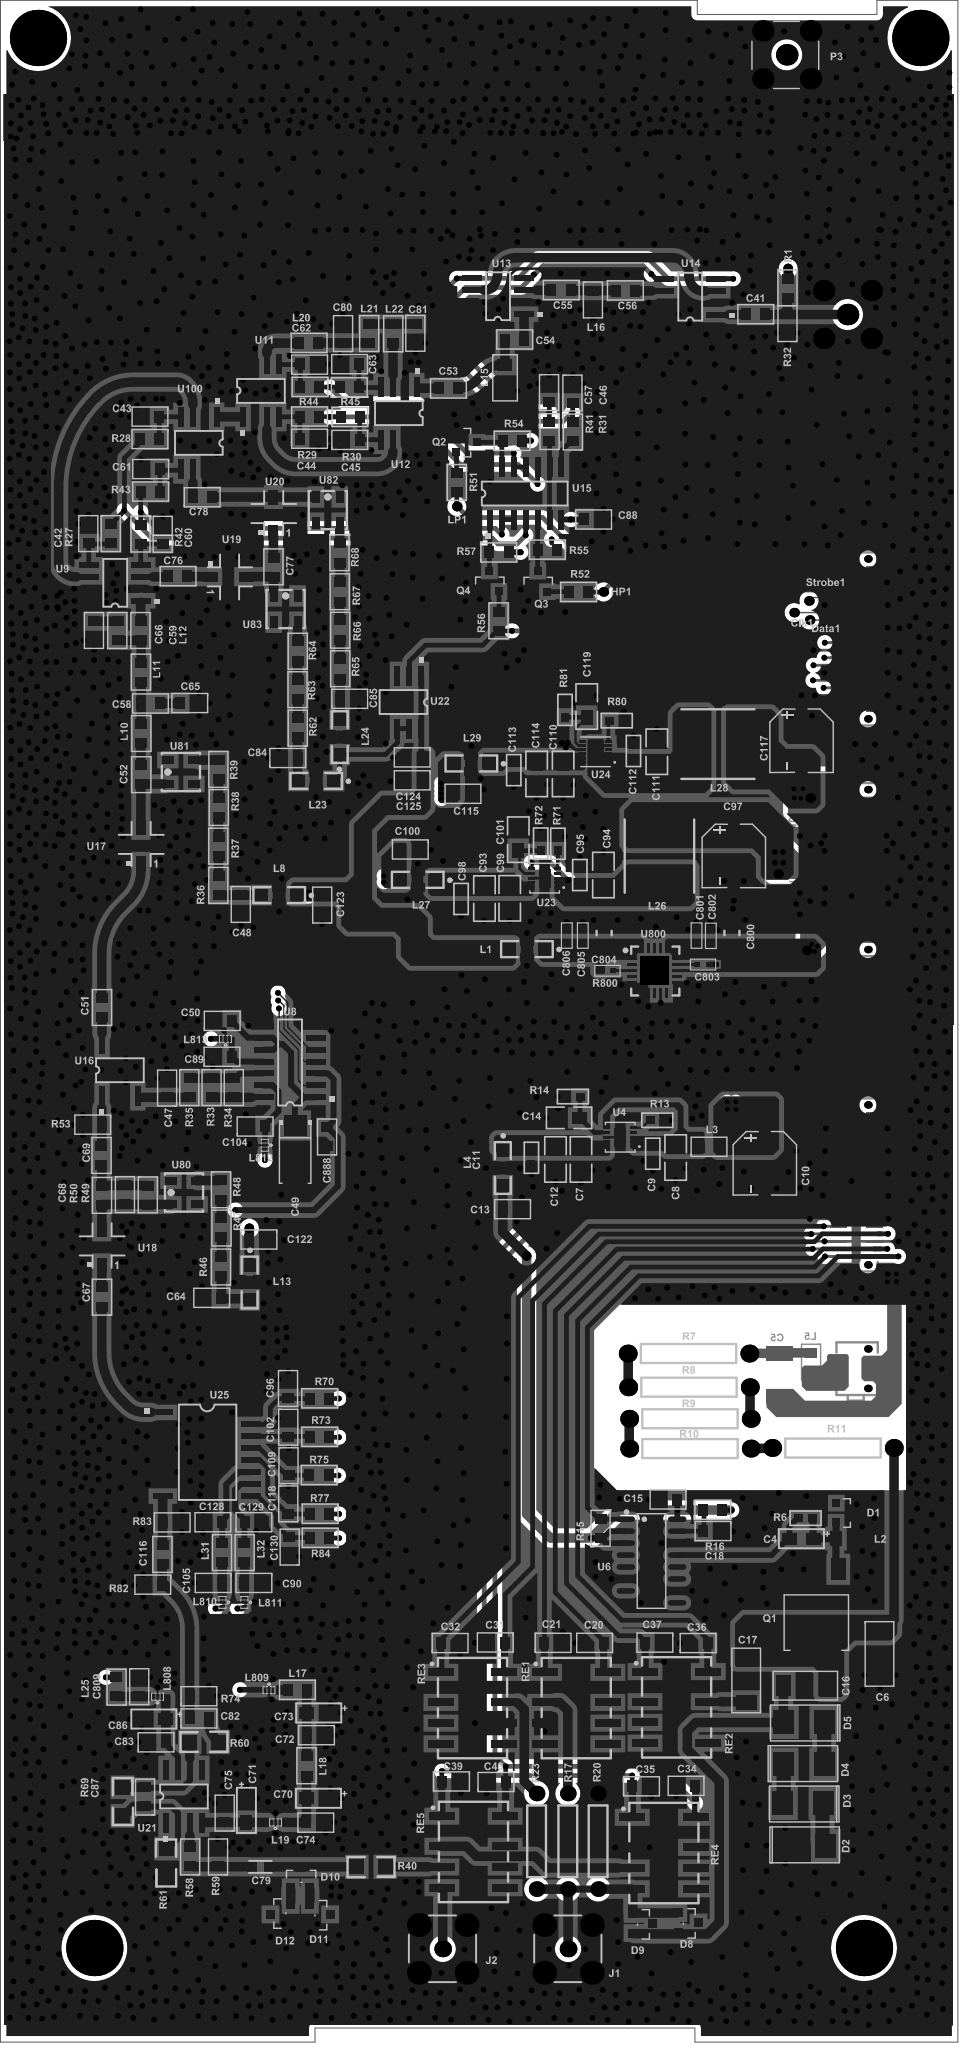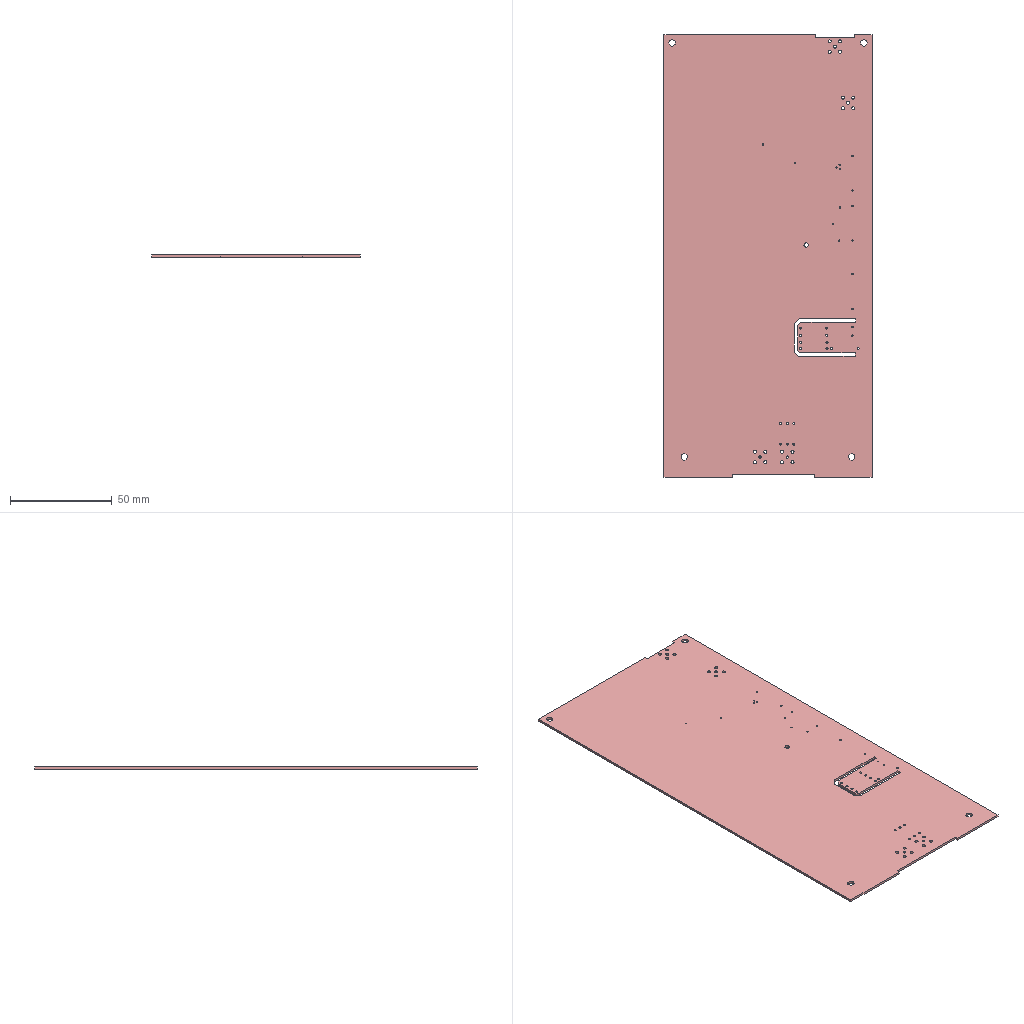Circuit board layout | Altium Designer | box 102 x 217 x 1.1 mm
Layer stack:
# Altium Designer layer stack of 10 (unit mm; dielectric type: 0 none, 1 core, 2 prepreg, 3 surface material)
index,name,kind,layer,copper_thickness_mm,dielectric_type,dielectric_thickness_mm,dielectric_material,dielectric_constant
0,TopPaste,other,,,,,,
1,TopOverlay,other,,,,,,
2,TopSolder,dielectric,,,3,0.0102,Solder Resist,3.5
3,TopLayer,copper,TopLayer,0.0356,,,,
4,Dielectric1,dielectric,,,1,0.32,FR-4,4.8
5,GND,copper,GND,0.0356,,,,
6,Dielectric3,dielectric,,,2,0.32,FR-4,4.8
7,SIG3,copper,SIG3,0.0356,,,,
8,Dielectric2,dielectric,,,1,0.32,FR-4,4.8
9,BottomLayer,copper,BottomLayer,0.0356,,,,
10,BottomSolder,dielectric,,,3,0.0102,Solder Resist,3.5
11,BottomOverlay,other,,,,,,
12,BottomPaste,other,,,,,,
# drill layer pairs: low layer,high layer
drill_pair,TopLayer,BottomLayer
Part placement:
Designator,Comment,Layer,Footprint,Center-X(mm),Center-Y(mm),Rotation
R1,0R,TopLayer,0805R,11.43,-30.582,90
+1,,BottomLayer,DIP-1,13.843,-84.785,360
+2,,BottomLayer,DIP-1,13.462,-100.965,360
1,,BottomLayer,DIP-1,10.414,-92.845,270
C71,25V 1UF Type A,TopLayer,0805C-2,-46.24,-192.38,270
C72,100NF 10%,TopLayer,0805R,-38.798,-184.404,360
C73,25V 1UF Type A,TopLayer,0805C-2,-38.544,-182.016,180
C74,100NF 10%,TopLayer,0805R,-38.823,-193.65,180
C75,100NF 10%,TopLayer,0805R,-48.577,-192.634,270
C76,10NF 10%,TopLayer,0805R,-53.543,-61.222,360
C77,10NF 10%,TopLayer,0805R,-43.332,-60.231,90
C78,10NF 10%,TopLayer,0805R,-50.927,-52.789,180
C79,100NF 10%,TopLayer,0603C,-44.755,-198.374,180
C80,33PF 10%,TopLayer,0805R,-35.966,-35.39,270
C81,33PF 10%,TopLayer,0805R,-28.219,-35.415,90
C82,100NF 10%,TopLayer,0805R,-51.269,-182.575,180
C83,100NF 10%,TopLayer,0805R,-55.841,-185.115,180
C84,100NF 10%,TopLayer,0805R,-41.808,-80.5,180
C85,100NF 10%,TopLayer,0805R,-35.204,-74.209,180
C86,25V 1UF Type A,TopLayer,0805C-2,-56.115,-182.662,180
C87,3pF( ±0.1pF),TopLayer,0805R,-57.061,-190.932,270
C88,100NF 10%,TopLayer,0805R,-9.22,-55.151,180
C89,100NF 10%,TopLayer,0805R,-48.818,-112.25,180
C90,100NF 10%,TopLayer,0805R,-45.464,-168.224,360
C93,22uF/16V,TopLayer,0805,-20.879,-95.461,90
C94,22uF/16V,TopLayer,0805,-8.204,-92.964,270
C95,100NF 10%,TopLayer,0603,-10.719,-92.964,90
C96,100NF 10%,TopLayer,0805R,-41.78,-147.559,90
C98,100NF 10%,TopLayer,0603,-23.368,-95.504,270
C99,22uF/16V,TopLayer,0805,-18.186,-95.436,90
C100,100NF 10%,TopLayer,0805R,-28.804,-90.272,360
C101,22uF  16V,TopLayer,0805,-17.272,-89.205,90
C102,100NF 10%,TopLayer,0805R,-41.755,-151.674,90
C103,100NF 10%,BottomLayer,0805R,13.818,-93.835,90
C104,100NF 10%,TopLayer,0805R,-45.287,-119.667,180
C105,100NF 10%,TopLayer,0805R,-49.808,-168.224,360
C106,100NF 10%,BottomLayer,0805R,13.818,-98.153,90
C107,100NF 10%,BottomLayer,0805R,13.868,-87.79,270
C109,100NF 10%,TopLayer,0805R,-41.729,-155.763,90
C110,22uF/16V,TopLayer,0805,-12.497,-82.22,90
C111,22uF/16V,TopLayer,0805,-2.515,-79.858,270
C112,100NF 10%,TopLayer,0603,-5.004,-79.781,90
C113,100NF 10%,TopLayer,0603,-17.755,-81.813,270
C114,22uF/16V,TopLayer,0805,-15.316,-82.22,90
C115,100NF 10%,TopLayer,0805R,-23.139,-84.303,180
C116,100NF 10%,TopLayer,0805R,-55.161,-165.194,90
C118,100NF 10%,TopLayer,0805R,-41.756,-159.817,90
C119,22uF  16V,TopLayer,0805,-9.982,-75.057,90
C122,100NF 10%,TopLayer,0805R,-44.926,-131.724,360
C123,100NF 10%,TopLayer,0805R,-38.187,-96.129,270
C124,100NF 10%,TopLayer,0805R,-28.6,-80.485,360
C125,100NF 10%,TopLayer,0805R,-28.6,-82.923,360
C128,100NF 10%,TopLayer,0805R,-49.833,-161.773,360
C129,100NF 10%,TopLayer,0805R,-45.413,-161.722,180
C130,100NF 10%,TopLayer,0805R,-41.654,-164.364,270
Clk1,,TopLayer,DIP-1,12.116,-65.075,270
D2,GF1M-E3/67A/GM,TopLayer,1808D,13.341,-196.113,180
D3,GF1M-E3/67A/GM,TopLayer,1808D,13.081,-191.618,360
D4,GF1M-E3/67A/GM,TopLayer,1808D,13.157,-187.477,180
D5,GF1M-E3/67A/GM,TopLayer,1808D,13.183,-183.007,360
D8,BAV99/A7,TopLayer,SOT-23-2,0.8509,-204.292,270
D9,BAV99/A7,TopLayer,SOT-23-2,-4.026,-204.394,270
D10,BAV99/A7,TopLayer,SOT-23-2,-40.494,-199.471,360
D11,BAV99/A7,TopLayer,SOT-23-2,-38.399,-203.421,270
D12,BAV99/A7,TopLayer,SOT-23-2,-42.595,-203.429,90
Data1,,TopLayer,DIP-1,13.767,-65.862,270
HP1,,TopLayer,DIP-1,-8.204,-62.873,270
L13,YFF31HC2A105MT000N,TopLayer,FILTER-SMD_4P-L3.2-W1.6-L_YFF31HC,-45.898,-136.267,270
L15,4.7UH 5%,TopLayer,1005L,-18.694,-40.107,270
L18,BLM21PG221SN1D(220O@100MHz,TopLayer,0805R,-39.814,-187.655,90
L25,BLM21PG221SN1D(220O@100MHz,TopLayer,0805R,-60.096,-179.248,270
L27,YFF31HC2A105MT000N,TopLayer,FILTER-SMD_4P-L3.2-W1.6-L_YFF31HC,-27.987,-93.472,180
L29,YFF31HC2A105MT000N,TopLayer,FILTER-SMD_4P-L3.2-W1.6-L_YFF31HC,-22.272,-81.102,180
L31,BLM21PG221SN1D(220O@100MHz,TopLayer,0805R,-48.817,-164.999,90
L32,BLM21PG221SN1D(220O@100MHz,TopLayer,0805R,-46.455,-164.948,270
LP1,,TopLayer,DIP-1,-23.825,-53.797,180
P5,Header 20X2,BottomLayer,N0.8mm/40Pin-Plug,18.726,-92.384,270
P6,RF connector SMB-JWHD SMB right-angle male plug, extended,BottomLayer,DIP-P-2,17.805,-33.393,180
Q4,MMBT3906/2A,TopLayer,SOT-23,-20.345,-61.73,360
R15,4.99K 1%,TopLayer,0805R,-8.484,-162.415,90
R16,2K 1%,TopLayer,0805R,3.424,-160.447,360
R53,10K 1%,TopLayer,0805R,-62.635,-119.515,360
R54,10K 1%,TopLayer,0805R,-17.907,-46.795,180
R55,10K 1%,TopLayer,0805R,-14.199,-58.402,360
R56,10K 1%,TopLayer,0805R,-19.355,-65.972,90
R57,10K 1%,TopLayer,0805R,-19.329,-58.656,180
R58,49.9R 1%,TopLayer,0805R,-52.259,-197.292,270
R59,4.99K 1%,TopLayer,0805R,-49.287,-197.292,270
R60,49.9R 1%,TopLayer,R-SMD_L3.5-W1.5,-50.758,-185.107,360
R61,30R 1%,TopLayer,R-SMD_L3.5-W1.5,-54.774,-197.959,90
R62,169R 1%,TopLayer,0805R,-40.792,-77.325,270
R63,169R 1%,TopLayer,0805R,-40.767,-73.287,90
R64,169R 1%,TopLayer,0805R,-40.792,-69.147,270
R65,49.9R 1%,TopLayer,0805R,-36.22,-71.059,90
R66,49.9R 1%,TopLayer,0805R,-36.271,-66.919,270
R67,49.9R 1%,TopLayer,0805R,-36.271,-62.881,90
R68,49.9R 1%,TopLayer,0805R,-36.297,-58.733,90
R69,120R 1%,TopLayer,R-SMD_L3.5-W1.5,-59.423,-191.433,270
R70,169R 1%,TopLayer,0805R,-38.453,-148.601,360
R71,0R1%,TopLayer,0603,-13.056,-89.637,90
R72,49.9K 1%,TopLayer,0603,-14.884,-89.611,90
R73,169R 1%,TopLayer,0805R,-38.453,-152.69,360
R74,NC,TopLayer,0805R,-51.269,-180.213,180
R75,169R 1%,TopLayer,0805R,-38.504,-156.754,360
R77,169R 1%,TopLayer,0805R,-38.403,-160.858,360
R80,0R1%,TopLayer,0603,-6.782,-76.556,360
R81,49.9K 1%,TopLayer,0603,-12.294,-75.413,90
R82,100K 1%,TopLayer,0805R,-56.236,-168.402,360
R83,10K 1%,TopLayer,0805R,-54.12,-161.739,180
R84,169R 1%,TopLayer,0805R,-38.403,-163.424,360
RE2,#NAME?,TopLayer,RELAY-SMD_PANASONIC_AGQ2X0AXX,-0.4061,-181.422,270
RE3,#NAME?,TopLayer,RELAY-SMD_PANASONIC_AGQ2X0AXX,-22.148,-181.498,270
RE4,#NAME?,TopLayer,RELAY-SMD_PANASONIC_AGQ2X0AXX,-1.761,-196.906,270
RE5,#NAME?,TopLayer,RELAY-SMD_PANASONIC_AGQ2X0AXX,-22.047,-196.789,270
Strobe1,,TopLayer,DIP-1,13.691,-63.83,270
U18,MAR-6SM/A06,TopLayer,LCC4,-61.644,-132.53,90
U19,MAR-6SM/A06,TopLayer,LCC4,-48.184,-61.247,360
U20,MAR-3SM/A03,TopLayer,LCC4,-43.358,-54.694,90
U21,MAX4106ESA+T,TopLayer,SO-8,-52.894,-190.866,90
U22,MIC4420CM,TopLayer,SO-8,-29.507,-74.6,270
U25,AT65-0263,TopLayer,SO-16,-50.437,-154.526,360
U100,SW-239,TopLayer,SO-8,-51.307,-47.059,270
C4,20PF 10%,TopLayer,0805C-2,12.878,-163.5,180
C5,330PF 10%,BottomLayer,1812C,10.516,-146.109,90
C6,22PF 10%,TopLayer,1812C-2,21.209,-175.717,270
C7,22uF/16V,TopLayer,0805,-10.592,-123.19,90
C8,22uF/16V,TopLayer,0805,-0.508,-122.987,90
C9,100NF 10%,TopLayer,0603,-2.946,-122.58,270
C11,100NF 10%,TopLayer,0603,-15.875,-123.012,270
C12,22uF/16V,TopLayer,0805,-13.31,-123.19,90
C13,100NF 10%,TopLayer,0805R,-17.907,-128.499,360
C14,22uF  16V,TopLayer,0805,-11.862,-118.77,180
C15,100NF 10%,TopLayer,0805R,-1.346,-159.352,360
C16,47PF 10%,TopLayer,1812C-2,13.284,-179.121,360
C17,100PF 10%,TopLayer,1812C-2,7.01,-178.587,90
C18,20PF 10%,TopLayer,0805R,3.449,-162.708,360
C20,100NF 10%,TopLayer,0805R,-9.169,-174.589,360
C21,100NF 10%,TopLayer,0805R,-13.538,-174.538,180
C31,100NF 10%,TopLayer,0805R,-19.753,-174.549,360
C32,100NF 10%,TopLayer,0805R,-24.511,-174.564,180
C34,100NF 10%,TopLayer,0805R,0.5776,-189.789,360
C35,100NF 10%,TopLayer,0805R,-4.121,-189.789,180
C36,100NF 10%,TopLayer,0805R,1.905,-174.564,180
C37,100NF 10%,TopLayer,0805R,-2.743,-174.564,360
C39,100NF 10%,TopLayer,0805R,-24.409,-189.321,360
C40,100NF 10%,TopLayer,0805R,-19.633,-189.332,180
C41,100NF 10%,TopLayer,0805R,8.001,-33.383,360
C42,100NF 10%,TopLayer,0805R,-63.058,-56.7,90
C43,100NF 10%,TopLayer,0805R,-56.539,-44.265,360
C44,100NF 10%,TopLayer,0805R,-39.533,-46.618,360
C45,100NF 10%,TopLayer,0805R,-35.204,-46.693,180
C46,100NF 10%,TopLayer,0805R,-11.481,-41.765,90
C47,100NF 10%,TopLayer,0805R,-54.711,-115.578,270
C48,100NF 10%,TopLayer,0805R,-46.812,-96.114,90
C49,22uF 25V,TopLayer,CAP-SMD_L6.0-W3.2-R-RD,-41.046,-122.544,90
C50,100NF 10%,TopLayer,0805R,-48.792,-108.44,180
C51,100NF 10%,TopLayer,0805R,-61.645,-107.018,270
C52,100NF 10%,TopLayer,0805R,-57.455,-82.271,270
C53,3.3NF 10%,TopLayer,0805R,-24.689,-41.224,180
C54,100NF 10%,TopLayer,0805R,-17.678,-36.068,360
C55,330PF 10%,TopLayer,0805R,-12.724,-30.812,360
C56,330PF 10%,TopLayer,0805R,-5.893,-30.853,360
C57,100NF 10%,TopLayer,0805R,-13.97,-41.715,90
C58,33PF 10%,TopLayer,0805R,-56.439,-74.709,180
C59,33PF 10%,TopLayer,0805R,-59.968,-66.998,90
C60,100NF 10%,TopLayer,0805R,-55.133,-56.776,90
C61,100NF 10%,TopLayer,0805R,-56.464,-49.843,360
C62,100NF 10%,TopLayer,0805R,-39.482,-38.693,180
C63,100NF 10%,TopLayer,0805R,-35.266,-38.693,360
C64,100NF 10%,TopLayer,0805R,-49.962,-137.921,360
C65,33PF 10%,TopLayer,0805R,-52.299,-74.709,360
C66,33PF 10%,TopLayer,0805R,-62.458,-66.998,90
C67,100NF 10%,TopLayer,0805R,-61.645,-137.803,270
C68,39PF 10%,TopLayer,0805R,-61.645,-126.982,270
C69,100NF 10%,TopLayer,0805R,-61.696,-122.741,270
C70,25V 1UF Type A,TopLayer,0805C-2,-38.569,-191.084,180
D1,BAV99/A7,TopLayer,SOT-23,17.678,-160.731,270
J1,RF connector,TopLayer,DIP-P,-11.97,-207.094,90
J2,RF connector,TopLayer,DIP-P,-25.324,-207.094,90
L2,15UH 5%,TopLayer,1005R,17.978,-163.482,360
L4,YFF31HC2A105MT000N,TopLayer,FILTER-SMD_4P-L3.2-W1.6-L_YFF31HC,-18.923,-124.1,270
L5,6.8UH 10%,BottomLayer,0805R,13.894,-144.762,90
L8,YFF31HC2A105MT000N,TopLayer,FILTER-SMD_4P-L3.2-W1.6-L_YFF31HC,-42.744,-95.098,180
L10,10NH 10%,TopLayer,0805R,-57.454,-77.895,270
L11,10NH 10%,TopLayer,0805R,-57.454,-71.418,90
L12,10NH 10%,TopLayer,0805R,-57.505,-66.998,90
L16,1UH 5%,TopLayer,0805R,-9.296,-31.869,90
L17,BLM21PG221SN1D(220O@100MHz),TopLayer,0805R,-40.83,-179.578,360
L19,NFM15PC104R1A3D,TopLayer,FILTER-SMD_0402-3P-L1.0-W0.5-T,-43.136,-193.65,180
L20,10NH 10%,TopLayer,0805R,-39.584,-36.432,360
L21,10NH 10%,TopLayer,0805R,-33.183,-35.391,270
L22,10NH 10%,TopLayer,0805R,-30.617,-35.416,270
L24,YFF31HC2A105MT000N,TopLayer,FILTER-SMD_4P-L3.2-W1.6-L_YFF31HC,-36.297,-78.303,90
P1,Header 20X2,BottomLayer,N0.8mm/40Pin-Plug,18.726,-125.896,270
P2,Header 4X2,BottomLayer,N0.8mm/8Pin-SOCKET,18.726,-145.427,270
P4,Header 20X2,BottomLayer,N0.8mm/40Pin-Plug,18.726,-67.87,270
Q1,MJD31C,TopLayer,SOT-252-2,14.402,-170.434,180
Q2,MMBT3906/2A,TopLayer,SOT-23,-22.773,-46.971,270
Q3,MMBT3906/2A,TopLayer,SOT-23,-15.189,-61.755,360
R6,2K 5%,TopLayer,0603,13.335,-161.315,180
R7,NC,TopLayer,AXIAL-0.51,0.8636,-143.823,180
R8,3.9K 5% 1/2W,TopLayer,AXIAL-0.51,0.9144,-147.404,180
R9,3.9K 5% 1/2W,TopLayer,AXIAL-0.51,1.016,-150.757,180
R10,3.9K 5% 1/2W,TopLayer,AXIAL-0.51,1.022,-153.922,180
R11,3.9K 5% 1/2W,TopLayer,AXIAL-0.51,16.256,-153.856,360
R13,0R1%,TopLayer,0603,-2.464,-119.024,360
R14,49.9K 1%,TopLayer,0603,-11.455,-116.51,180
R17,49.9R 1% 1/4W,TopLayer,AXIAL-0.4,-11.995,-195.656,90
R20,100R 1% 1/4W,TopLayer,AXIAL-0.4,-8.77,-195.656,90
R23,100R 1% 1/4W,TopLayer,AXIAL-0.4,-15.323,-195.656,90
R27,4.87K 1%,TopLayer,0805R,-60.67,-56.7,90
R28,4.87K 1%,TopLayer,0805R,-56.539,-46.653,360
R29,4.87K 1%,TopLayer,0805R,-39.533,-44.252,360
R30,4.87K 1%,TopLayer,0805R,-35.189,-44.256,180
R31,4.87K 1%,TopLayer,0805R,-11.481,-45.855,270
R32,10K 1%,TopLayer,0805R,11.379,-34.333,270
R33,100K 1%,TopLayer,0805R,-49.921,-115.578,90
R34,100K 1%,TopLayer,0805R,-47.558,-115.579,90
R35,49.9R 1%,TopLayer,0805R,-52.298,-115.578,90
R36,49.9R 1%,TopLayer,0805R,-49.207,-94.082,90
R37,49.9R 1%,TopLayer,0805R,-49.207,-89.916,90
R38,49.9R 1%,TopLayer,0805R,-49.207,-85.761,270
R39,49.9R 1%,TopLayer,0805R,-49.2,-81.763,90
R40,49.9R 1% 1/4W,TopLayer,R-SMD_L3.5-W1.5,-32.963,-198.374,180
R41,10K 1%,TopLayer,0805R,-13.97,-45.804,270
R42,4.87K 1%,TopLayer,0805R,-57.495,-56.75,90
R43,4.87K 1%,TopLayer,0805R,-56.464,-52.23,360
R44,4.87K 1%,TopLayer,0805R,-39.482,-41.106,360
R45,4.87K 1%,TopLayer,0805R,-35.255,-41.105,180
R46,169R 1%,TopLayer,0805R,-48.971,-134.595,270
R47,169R 1%,TopLayer,0805R,-48.92,-130.454,270
R48,169R 1%,TopLayer,0805R,-48.92,-126.441,90
R49,49.9R 1%,TopLayer,0805R,-56.717,-126.982,90
R50,49.9R 1%,TopLayer,0805R,-59.156,-126.957,90
R51,10K 1%,TopLayer,0805R,-23.851,-51.214,270
R52,10K 1%,TopLayer,0805R,-10.871,-62.898,360
RE1,#NAME?,TopLayer,RELAY-SMD_PANASONIC_AGQ2X0AXX,-11.099,-181.498,270
U6,74HCT123D,TopLayer,SOIC-16_L9.9-W3.9-P1.27-LS6.0-BL,-3.081,-165.87,270
U8,MAX504CSD+T,TopLayer,SO-14,-41.615,-112.785,180
U9,SW-239,TopLayer,SO-8,-60.238,-61.907,180
U11,SW-239,TopLayer,SO-8,-44.689,-41.487,90
U12,SW-239,TopLayer,SO-8,-29.997,-43.899,270
U13,SW-239,TopLayer,SO-8,-19.455,-31.447,180
U14,SW-239,TopLayer,SO-8,1.017,-31.498,180
U15,74HCT04D,TopLayer,SO-14,-16.484,-52.393,90
U16,AT-250(MAAV-007941),TopLayer,SO-8,-59.713,-113.683,90
U17,MAR-3SM/A03,TopLayer,LCC4,-57.479,-89.858,90
C10,220UF 25V (D6.3*7.7mm),TopLayer,CAP-SMD_BD6.3-L6.6-W6.6-FD,8.992,-123.6,270
C97,220UF 25V (D6.3*7.7mm),TopLayer,CAP-SMD_BD6.3-L6.6-W6.6-FD,5.69,-90.935,270
C117,220UF 25V (D6.3*7.7mm),TopLayer,CAP-SMD_BD6.3-L6.6-W6.6-FD,12.903,-78.692,270
L3,BLM21PG221SN1D(220O@100MHz),TopLayer,0805R,3.073,-121.818,180
L26,CD75-470M(47uH/1A),TopLayer,IND-SMD_L7.8-W7.0-A,-2.235,-90.95,90
L28,CD75-470M(47uH/1A),TopLayer,IND-SMD_L7.8-W7.0-A,3.995,-79.045,360
U4,LT3045EDD#PBF,TopLayer,DFN-10_L3.0-W3.0-P0.50-BL-EP,-6.415,-120.826,90
U23,LT3045EDD#PBF,TopLayer,DFN-10_L3.0-W3.0-P0.50-BL-EP,-14.467,-93.293,90
U24,LT3094EDD#PBF,TopLayer,WDFN-12_L3.0-W3.0-P0.45-BL-EP,-9.042,-79.865,90
L23,YFF31HC2A105MT000N,TopLayer,FILTER-SMD_4P-L3.2-W1.6-L_YFF31HC,-38.807,-82.956,180
C800,47uF 25V,TopLayer,1206,5.588,-99.136,180
C801,0.1uF,TopLayer,0402,1.702,-99.398,90
C802,1uF 25V,TopLayer,0402,3.226,-99.423,90
C803,1uF 25V,TopLayer,0402,2.413,-102.464,360
C804,47uF 25V,TopLayer,1206,-8.026,-99.144,180
C805,0.1uF,TopLayer,0402,-10.414,-99.398,90
C806,1uF 25V,TopLayer,0402,-12.116,-99.398,90
L1,YFF31HC2A105MT000N,TopLayer,FILTER-SMD_4P-L3.2-W1.6-L_YFF31HC,-16.353,-100.838,180
L808,NFM15PC104R1A3D,TopLayer,FILTER-SMD_0402-3P-L1.0-W0.5-T,-55.709,-180.289,180
L809,NFM15PC104R1A3D,TopLayer,FILTER-SMD_0402-3P-L1.0-W0.5-T,-43.834,-179.578,360
L810,NFM15PC104R1A3D,TopLayer,FILTER-SMD_0402-3P-L1.0-W0.5-T,-48.793,-170.263,270
L811,NFM15PC104R1A3D,TopLayer,FILTER-SMD_0402-3P-L1.0-W0.5-T,-46.457,-170.263,270
L812,NFM15PC104R1A3D,TopLayer,FILTER-SMD_0402-3P-L1.0-W0.5-T,-44.271,-121.68,270
L813,NFM15PC104R1A3D,TopLayer,FILTER-SMD_0402-3P-L1.0-W0.5-T,-48.47,-110.388,180
R800,0R,TopLayer,0402,-7.772,-103.124,360
U800,TPS7A4701RGWR,TopLayer,QFN-20,-2.756,-103.111,360
P3,RF connector SMB-JWHD SMB right-angle male plug, extended,TopLayer,DIP-P-2,11.328,-5.791,90
C809,100nF 10%,TopLayer,0805R,-57.633,-179.248,90
C888,100nF 10%,TopLayer,0805R,-37.668,-120.777,270
U80,TCCH-80+,TopLayer,IND-SMD_4P-L3.8-W3.8,-52.884,-126.703,90
U81,TCCH-80+,TopLayer,IND-SMD_4P-L3.8-W3.8,-53.215,-82.017,90
U82,TCCH-80+,TopLayer,IND-SMD_4P-L3.8-W3.8,-37.567,-54.176,0
U83,TCCH-80+,TopLayer,IND-SMD_4P-L3.8-W3.8,-42.062,-64.692,0
Pad and via stacks:
# Altium Designer via and pad stacks of 10 (unit mm). Each distinct definition once, with the count of objects using it.
# via: kind,start_layer,end_layer,hole_mm,diameter_mm,mode(0 simple;1 top-mid-bottom;2 full stack),diameter_per_layer,count,example_net
# pad: kind,layer,hole_mm,hole_type(0 round;1 square;2 slot),plating,top_size,top_shape(1 round;2 rect;3 octagon;9 rounded rect),mid_size,bottom_size,mode,footprint,size_per_layer,count,example
pad,TopLayer,0,0,plated,1.5x1.566,2,1.5x1.566,1.5x1.566,0,R-SMD_L3.5-W1.5,,8,R40.1
pad,TopLayer,0,0,plated,0.3048x1.016,2,0.3048x1.016,0.3048x1.016,0,QFN-20,,20,U800.2
pad,TopLayer,0,0,plated,0.15x0.46,2,0.15x0.46,0.15x0.46,0,FILTER-SMD_0402-3P-L1.0-W0.5-T,,14,L808.1
pad,TopLayer,0,0,plated,0.15x0.2,2,0.15x0.2,0.15x0.2,0,FILTER-SMD_0402-3P-L1.0-W0.5-T,,14,L808.2
pad,TopLayer,0,0,plated,0.635x0.508,2,0.635x0.508,0.635x0.508,0,0402,,12,C801.2
pad,TopLayer,0,0,plated,1.829x1.575,2,1.829x1.575,1.829x1.575,0,1206,,4,C800.1
pad,TopLayer,0,0,plated,0.252x0.665,2,0.252x0.665,0.252x0.665,0,WDFN-12_L3.0-W3.0-P0.45-BL-EP,,12,U24.1
pad,TopLayer,0,0,plated,2.4x1.7,2,2.4x1.7,2.4x1.7,0,WDFN-12_L3.0-W3.0-P0.45-BL-EP,,1,U24.13
pad,TopLayer,0,0,plated,0.25x0.65,2,0.25x0.65,0.25x0.65,0,DFN-10_L3.0-W3.0-P0.50-BL-EP,,20,U4.1
pad,TopLayer,0,0,plated,2x1.2,2,2x1.2,2x1.2,0,DFN-10_L3.0-W3.0-P0.50-BL-EP,,2,U4.11
pad,TopLayer,0,0,plated,3.5x7,2,3.5x7,3.5x7,0,IND-SMD_L7.8-W7.0-A,,4,L26.1
pad,TopLayer,0,0,plated,3.5x1.2,2,3.5x1.2,3.5x1.2,0,CAP-SMD_BD6.3-L6.6-W6.6-FD,,6,C10.1
pad,TopLayer,0,0,plated,2.032x0.635,2,2.032x0.635,2.032x0.635,0,SO-14,,28,U8.6
pad,TopLayer,0,0,plated,0.602x1.971,1,0.602x1.971,0.602x1.971,0,SOIC-16_L9.9-W3.9-P1.27-LS6.0-BL,,16,U6.1
pad,TopLayer,0,0,plated,0.889x0.889,2,0.889x0.889,0.889x0.889,0,0603R,,2,R6.1
pad,TopLayer,0,0,plated,2.286x1.524,2,2.286x1.524,2.286x1.524,0,SOT-252-2,,2,Q1.2
pad,TopLayer,0,0,plated,4.826x5.08,2,4.826x5.08,4.826x5.08,0,SOT-252-2,,1,Q1.3
pad,TopLayer,0,0,plated,1.27x1.524,2,1.27x1.524,1.27x1.524,0,1005R,,2,L2.2
pad,TopLayer,0,0,plated,2.208x2.376,2,2.208x2.376,2.208x2.376,0,CAP-SMD_L6.0-W3.2-R-RD,,2,C49.1
pad,TopLayer,0,0,plated,1.524x2.159,2,1.524x2.159,1.524x2.159,0,1812C-2,,6,C6.1
pad,TopLayer,0,0,plated,1.27x1.016,2,1.27x1.016,1.27x1.016,0,0805C,,2,C4.1
pad,TopLayer,0,0,plated,2.032x0.635,2,2.032x0.635,2.032x0.635,0,SO-16,,16,U25.16
pad,TopLayer,0,0,plated,2.032x0.635,2,2.032x0.635,2.032x0.635,0,SO-8,,72,U21.3
pad,TopLayer,0,0,plated,1.524x1.016,2,1.524x1.016,1.524x1.016,0,LCC4,,16,U18.2
pad,TopLayer,0,0,plated,0.8x2.7,2,0.8x2.7,0.8x2.7,0,RELAY-SMD_PANASONIC_AGQ2X0AXX,,40,RE2.8
pad,TopLayer,0,0,plated,0.762x0.762,2,0.762x0.762,0.762x0.762,0,SOT-23,,12,Q4.1
pad,TopLayer,0,0,plated,1.524x1.27,2,1.524x1.27,1.524x1.27,0,1005L,,2,L15.2
pad,TopLayer,0,0,plated,1.4x0.9,2,1.4x0.9,1.4x0.9,0,FILTER-SMD_4P-L3.2-W1.6-L_YFF31HC,,16,L13.4
pad,TopLayer,0,0,plated,1.3x1.2,2,1.3x1.2,1.3x1.2,0,FILTER-SMD_4P-L3.2-W1.6-L_YFF31HC,,16,L13.3
pad,TopLayer,0,0,plated,0.889x0.889,2,0.889x0.889,0.889x0.889,0,SOT-23-2,,15,D8.3
pad,TopLayer,0,0,plated,2.54x2.159,2,2.54x2.159,2.54x2.159,0,1808D,,8,D2.2
pad,TopLayer,0,0,plated,0.889x0.762,2,0.889x0.762,0.889x0.762,0,0603,,22,C95.1
pad,TopLayer,0,0,plated,1.524x1.27,2,1.524x1.27,1.524x1.27,0,0805,,24,C93.2
pad,TopLayer,0,0,plated,1.016x1.016,2,1.016x1.016,1.016x1.016,0,0603C,,2,C79.2
pad,TopLayer,0,0,plated,1.27x1.016,2,1.27x1.016,1.27x1.016,0,0805R,,274,C72.1
pad,TopLayer,0,0,plated,1.27x1.524,2,1.27x1.524,1.27x1.524,0,0805C-2,,8,C71.2
pad,TopLayer,0,0,plated,0.76x1.27,2,0.76x1.27,0.76x1.27,0,IND-SMD_4P-L3.8-W3.8,,16,U82.3
pad,MultiLayer,1.524,0,plated,2.286x2.286,1,2.286x2.286,2.286x2.286,0,DIP-P-2,,10,P3.5
pad,MultiLayer,1.524,0,plated,2.54x2.54,1,2.54x2.54,2.54x2.54,0,DIP-P,,8,J2.1
pad,MultiLayer,1.143,0,plated,1.778x1.778,1,1.778x1.778,1.778x1.778,0,DIP-P,,2,J2.5
pad,MultiLayer,0.68,0,plated,0.8x0.8,1,0.8x0.8,0.8x0.8,0,N0.8mm/8Pin-SOCKET,,2,P2.0
pad,MultiLayer,0.68,0,plated,0.8x0.8,1,0.8x0.8,0.8x0.8,0,N0.8mm/40Pin-Plug,,6,P5.0
pad,MultiLayer,2.159,0,plated,3.048x3.048,2,3.048x3.048,3.048x3.048,0,QFN-20,,1,U800.21
pad,MultiLayer,1.016,0,plated,1.651x1.651,1,1.651x1.651,1.651x1.651,0,AXIAL-0.4,,6,R17.2
pad,MultiLayer,1.016,0,plated,1.905x1.905,1,1.905x1.905,1.905x1.905,0,AXIAL-0.51,,10,R7.1
pad,MultiLayer,0.635,0,plated,1.016x1.016,1,1.016x1.016,1.016x1.016,0,DIP-1,,8,Clk1.1
pad,MultiLayer,3.2,0,plated,6x6,1,6x6,6x6,0,,,4,0
pad,BottomLayer,0,0,plated,0.3x1.8,2,0.3x1.8,0.3x1.8,0,N0.8mm/8Pin-SOCKET,,8,P2.2
pad,BottomLayer,0,0,plated,2.794x1.524,2,2.794x1.524,2.794x1.524,0,1812C,,2,C5.1
pad,BottomLayer,0,0,plated,0.3x1.8,2,0.3x1.8,0.3x1.8,0,N0.8mm/40Pin-Plug,,120,P5.8
pad,BottomLayer,0,0,plated,0.889x0.762,2,0.889x0.762,0.889x0.762,0,0603,,4,C98.1
pad,BottomLayer,0,0,plated,1.27x1.016,2,1.27x1.016,1.27x1.016,0,0805R,,8,C107.1
via,TopLayer,BottomLayer,0.3048,0.6096,0,,2635,GND
via,TopLayer,BottomLayer,0.3048,0.508,0,,1,GND
via,TopLayer,BottomLayer,0.508,1.016,0,,1,NetC41_2
Copper pours:
name,layer,net,type(0 solid;1 hatched;2 none)
Bottom Layer-No Net,TopLayer,NetC6_1,0
Bottom Layer-No Net,TopLayer,GND,0
Bottom Layer-No Net,TopLayer,,0
Bottom Layer-No Net,BottomLayer,,0
Bottom Layer-No Net,BottomLayer,HT,0
Bottom Layer-No Net,BottomLayer,+12.5V,0
Bottom Layer-No Net,BottomLayer,A6V,0
Bottom Layer-No Net,BottomLayer,GND,0
Bottom Layer-No Net,BottomLayer,,0
Bottom Layer-No Net,SIG3,GND,0
Bottom Layer-No Net,SIG3,,0
Bottom Layer-No Net,GND,,0
Bottom Layer-No Net,GND,GND,0
Design rules, without the lines most boards share:
# Altium Designer design rules of 10 (exported by Altium Designer, unit mm)
# columns: name | kind | enabled | priority | scope1 | scope2 | descriptor | typed fields (field=value)
ComponentClearance | 24 | disabled | 1 | All | All | Component Clearance Constraint ( Horizontal Gap = 10mil, Vertical Gap = 10mil ) (Disabled)(All),(All)  | gap=0.254
HoleSize | 42 | disabled | 1 | All | All | Hole Size Constraint (Min=1mil) (Max=500mil) (Disabled)(All) |
Clearance_1 | 0 | disabled | 2 | (IsKeepOut) | All | Clearance Constraint (Gap=6mil) (Disabled)((IsKeepOut)),(All) | gap=0.1524
PlaneConnect | 6 | enabled | 1 | All | All | Power Plane Connect Rule(Direct Connect )(Expansion=20mil) (Conductor Width=10mil) (Air Gap=10mil) (Entries=4) (All) | relief_conductor_width=0.254 relief_entries=4 relief_expansion=0.508
PlaneClearance | 12 | enabled | 1 | All | All | Power Plane Clearance (Clearance =6mil) (All) | clearance=0.1524
PolygonConnect | 20 | enabled | 1 | All | All | Polygon Connect Rule(Direct Connect )(Conductor Width=10mil) (Relief Angle=90 Angle) (Entries=4) (Air Gap Width=10mil) (All),(All) | connect_style(0=relief,1=direct,2=none)=1 relief_conductor_width=0.254 relief_entries=4
Width | 2 | enabled | 1 | All | All | Width Constraint (Min=5mil) (Max=200mil) (Preferred=200mil) (All) |
RoutingVias | 11 | enabled | 1 | All | All | Routing Via (MinHoleWidth=12mil) (MaxHoleWidth=20mil) (PreferredHoleWidth=12mil) (MinWidth=20mil) (MaxWidth=40mil) (PreferedWidth=20mil) (All) | via_min_hole=0.3048 via_max_hole=0.508 via_preferred_diameter=0.508 via_preferred_hole=0.3048
SolderMaskExpansion | 13 | enabled | 1 | All | All | Solder Mask Expansion (Expansion =4mil) (All) | expansion=0.1016
TestPointUsage | 44 | enabled | 1 | All | All | Fabrication Testpoint Usage (Valid =One Required, Allow multiple per net=No) (All) |
Testpoint | 43 | enabled | 1 | All | All | Fabrication Testpoint Style (Under Component=Yes) (All) |
Clearance | 0 | enabled | 3 | All | All | Clearance Constraint (Gap=6mil) (All),(All) | gap=0.1524
DiffPairsRouting | 51 | enabled | 1 | All | All | Differential Pairs Uncoupled Length using the Gap Constraints (Min=6mil) (Max=6mil) (Prefered=6mil)  and Width Constraints (Min=15mil) (Max=15mil) (Prefered=15mil) (All) |
HoleToHoleClearance | 52 | enabled | 1 | All | All | Hole To Hole Clearance (Gap=0mil) (All),(All) | gap=0
MinimumSolderMaskSliver | 53 | enabled | 1 | All | All | Minimum Solder Mask Sliver (Gap=0mil) (All),(All) |
SilkscreenOverComponentPads | 54 | enabled | 1 | IsPad | All | Silk To Solder Mask (Clearance=0mil) (IsPad),(All) |
SilkToSilkClearance | 55 | enabled | 1 | All | All | Silk to Silk (Clearance=0mil) (All),(All) |
Clearance_2 | 0 | enabled | 1 | inpolygon | All | Clearance Constraint (Gap=6mil) (inpolygon),(All) | gap=0.1524
Classes set for this board:
# Altium Designer classes of 10 (member kind: 0 net, 1 component, 2 from-to, 3 pad, 4 layer, 5 differential pair, 6 design channel, 7 polygon, 8 structure, 9 xSignal)
# columns: class name | member kind | superclass | members
All From-Tos | 0 | yes |
JSR 1002010B | 1 | no | +1; +2; 1; C4; C5; C6; C7; C8; C9; C10; C11; C12; C13; C14; C15; C16; C17; C18; C20; C21; C31; C32; C34; C35; C36; C37; C39; C40; C41; C42; C43; C44; C45; C46; C47; C48; C49; C50; C51; C52; C53; C54; C55; C56; C57; C58; C59; C60; C61; C62; C63; C64; C65; C66; C67; C68; C69; C70; C71; C72; C73; C74; C75; C76; C77; C78; C79; C80; C81; C82; C83; C84; C85; C86; C87; C88; C89; C90; C93; C94; C95; C96; C97; C98; C99; C100; C101; C102; C103; C104; C105; C106; C107; C109; C110; C111; C112; C113; C114; C115; C116; C117; C118; C119; C122; C123; C124; C125; C128; C129; C130; Clk1; D1; D2; D3; D4; D5; D8; D9; D10; D11; D12; Data1; HP1; J1; J2; L2; L3; L4; L5; L8; L10; L11; L12; L13; L15; L16; L17; L18; L19; L20; L21; L22; L23; L24; L25; L26; L27; L28; L29; L31; L32; LP1; P1; P2; P3; P4; P5; P6; Q1; Q2; Q3; Q4; R6; R7; R8; R9; R10; R11; R13; R14; R15; R16; R17; R20; R23; R27; R28; R29; R30; R31; R32; R33; R34; R35; R36; R37; R38; R39; R40; R41; R42; R43; R44; R45; R46; R47; R48; R49; R50; R51; R52; R53; R54; R55; R56; R57; R58; R59; R60; R61; R62; R63; R64; R65; R66; R67; R68; R69; R70; R71; R72; R73; R74; R75; R77; R78; R80; R81; R82; R83; R84; RE1; RE2; RE3; RE4; RE5; Strobe1; U4; U6; U8; U9; U11; U12; U13; U14; U15; U16; U17; U18; U19; U20; U21; U22; U23; U24; U25; U100; C4; C5; C6; C7; C8; C9; C11; C12; C13; C14; C15; C16; C17; C18; C20; C21; C31; C32; C34; C35; C36; C37; C39; C40; C41; C42; C43; C44; C45; C46; C47; C48; C49; C50; C51; C52; C53; C54; C55; C56; C57; C58; C59; C60; C61; C62; C63; C64; C65; C66; C67; C68; C69; C70; D1; J1; J2; L2; L4; L5; L8; L10; L11; L12; L16; L17; L19; L20; L21; L22; L23; L24; P1; P2; P3; P4; Q1; Q2; Q3; R6; R7; R8; R9; R10; R11; R13; R14; R17; R20; R23; R27; R28; R29; R30; R31; R32; R33; R34; R35; R36; R37; R38; R39; R40; R41; R42; R43; R44; R45; R46; R47; R48; R49; R50; R51; R52; RE1; U6; U8; U9; U11; U12; U13; U14; U15; U16; U17; C10; C97; C117; L3; L26; L28; U4; U23; U24; C800; C801; C802; C803; C804; C805; C806; L1; L808; L809; L810; L811; L812; L813; R800; U800; C809; C888; U80; U81; U82; U83;